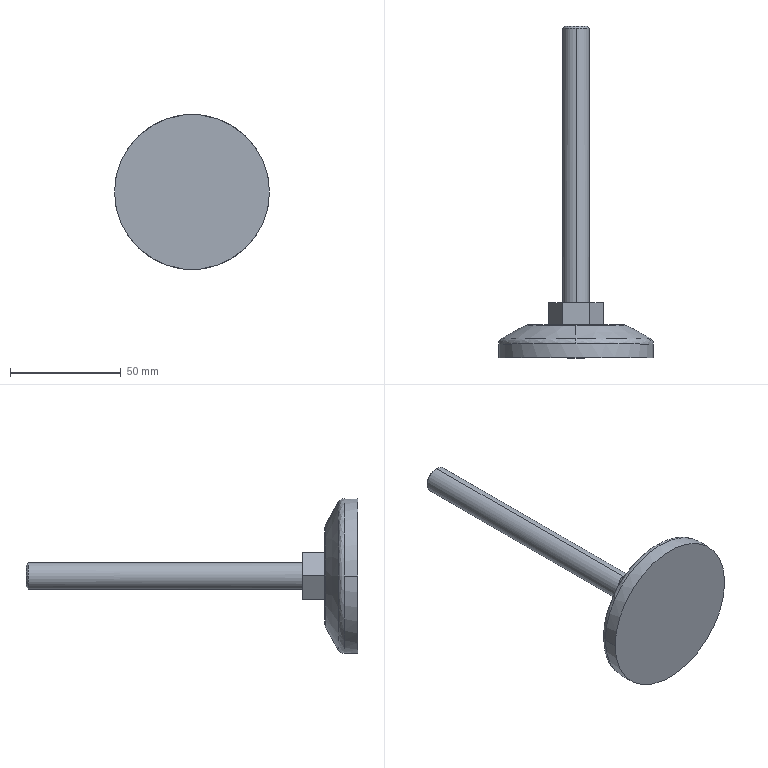Part | STEP file | Foot cup NFJNS16-130 | 1 solid | 22 faces | box 70 x 150 x 70 mm | volume 67181 mm3 | plane 10 | cone 4 | cylinder 4 | spline 4 | commonest cylinder face diameters 12 x2 70 x2